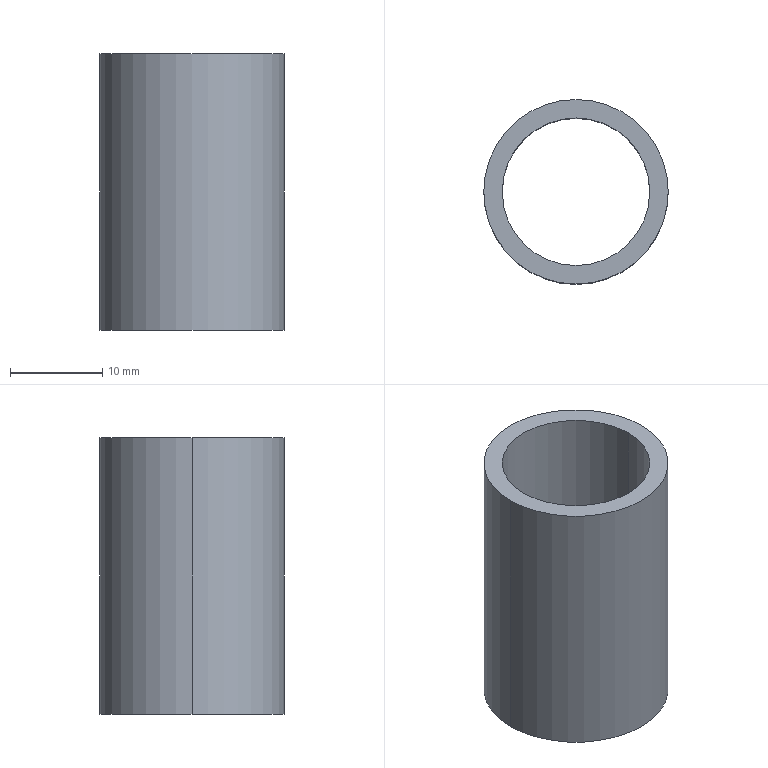Part | SolidWorks | features ExtruThin 1 | 1 solid | 6 faces | box 20 x 20 x 30 mm | volume 3393 mm3 | cylinder 4 | plane 2 | commonest cylinder face diameters 16 x2 20 x2
STEP:
#1=CARTESIAN_POINT('',(-8.,0.,30.));
#2=VERTEX_POINT('',#1);
#3=CARTESIAN_POINT('',(8.,0.,30.));
#4=VERTEX_POINT('',#3);
#5=CARTESIAN_POINT('',(0.,0.,30.));
#6=DIRECTION('',(0.,0.,1.));
#7=DIRECTION('',(1.,0.,0.));
#8=AXIS2_PLACEMENT_3D('',#5,#6,#7);
#9=CIRCLE('',#8,8.);
#10=EDGE_CURVE('',#2,#4,#9,.T.);
#11=ORIENTED_EDGE('',*,*,#10,.T.);
#12=CARTESIAN_POINT('',(8.,0.,0.));
#13=VERTEX_POINT('',#12);
#14=CARTESIAN_POINT('',(8.,0.,30.));
#15=DIRECTION('',(0.,0.,-1.));
#16=VECTOR('',#15,1000.);
#17=LINE('',#14,#16);
#18=EDGE_CURVE('',#4,#13,#17,.T.);
#19=ORIENTED_EDGE('',*,*,#18,.T.);
#20=CARTESIAN_POINT('',(-8.,0.,0.));
#21=VERTEX_POINT('',#20);
#22=CARTESIAN_POINT('',(0.,0.,0.));
#23=DIRECTION('',(0.,0.,1.));
#24=DIRECTION('',(1.,0.,0.));
#25=AXIS2_PLACEMENT_3D('',#22,#23,#24);
#26=CIRCLE('',#25,8.);
#27=EDGE_CURVE('',#21,#13,#26,.T.);
#28=ORIENTED_EDGE('',*,*,#27,.F.);
#29=CARTESIAN_POINT('',(-8.,0.,30.));
#30=DIRECTION('',(0.,0.,-1.));
#31=VECTOR('',#30,1000.);
#32=LINE('',#29,#31);
#33=EDGE_CURVE('',#2,#21,#32,.T.);
#34=ORIENTED_EDGE('',*,*,#33,.F.);
#35=EDGE_LOOP('',(#11,#19,#28,#34));
#36=FACE_OUTER_BOUND('',#35,.T.);
#37=CARTESIAN_POINT('',(0.,0.,30.));
#38=DIRECTION('',(0.,0.,-1.));
#39=DIRECTION('',(-1.,0.,0.));
#40=AXIS2_PLACEMENT_3D('',#37,#38,#39);
#41=CYLINDRICAL_SURFACE('',#40,8.);
#42=ADVANCED_FACE('',(#36),#41,.F.);
#43=CARTESIAN_POINT('',(10.,0.,30.));
#44=VERTEX_POINT('',#43);
#45=CARTESIAN_POINT('',(-10.,0.,30.));
#46=VERTEX_POINT('',#45);
#47=CARTESIAN_POINT('',(0.,0.,30.));
#48=DIRECTION('',(0.,0.,1.));
#49=DIRECTION('',(1.,0.,0.));
#50=AXIS2_PLACEMENT_3D('',#47,#48,#49);
#51=CIRCLE('',#50,10.);
#52=EDGE_CURVE('',#44,#46,#51,.T.);
#53=ORIENTED_EDGE('',*,*,#52,.F.);
#54=CARTESIAN_POINT('',(10.,0.,0.));
#55=VERTEX_POINT('',#54);
#56=CARTESIAN_POINT('',(10.,0.,30.));
#57=DIRECTION('',(0.,0.,-1.));
#58=VECTOR('',#57,1000.);
#59=LINE('',#56,#58);
#60=EDGE_CURVE('',#44,#55,#59,.T.);
#61=ORIENTED_EDGE('',*,*,#60,.T.);
#62=CARTESIAN_POINT('',(-10.,0.,0.));
#63=VERTEX_POINT('',#62);
#64=CARTESIAN_POINT('',(0.,0.,0.));
#65=DIRECTION('',(0.,0.,1.));
#66=DIRECTION('',(1.,0.,0.));
#67=AXIS2_PLACEMENT_3D('',#64,#65,#66);
#68=CIRCLE('',#67,10.);
#69=EDGE_CURVE('',#55,#63,#68,.T.);
#70=ORIENTED_EDGE('',*,*,#69,.T.);
#71=CARTESIAN_POINT('',(-10.,0.,30.));
#72=DIRECTION('',(0.,0.,-1.));
#73=VECTOR('',#72,1000.);
#74=LINE('',#71,#73);
#75=EDGE_CURVE('',#46,#63,#74,.T.);
#76=ORIENTED_EDGE('',*,*,#75,.F.);
#77=EDGE_LOOP('',(#53,#61,#70,#76));
#78=FACE_OUTER_BOUND('',#77,.T.);
#79=CARTESIAN_POINT('',(0.,0.,30.));
#80=DIRECTION('',(0.,0.,-1.));
#81=DIRECTION('',(-1.,0.,0.));
#82=AXIS2_PLACEMENT_3D('',#79,#80,#81);
#83=CYLINDRICAL_SURFACE('',#82,10.);
#84=ADVANCED_FACE('',(#78),#83,.T.);
#85=CARTESIAN_POINT('',(0.,0.,30.));
#86=DIRECTION('',(0.,0.,1.));
#87=DIRECTION('',(1.,0.,0.));
#88=AXIS2_PLACEMENT_3D('',#85,#86,#87);
#89=CIRCLE('',#88,10.);
#90=EDGE_CURVE('',#46,#44,#89,.T.);
#91=ORIENTED_EDGE('',*,*,#90,.T.);
#92=ORIENTED_EDGE('',*,*,#52,.T.);
#93=EDGE_LOOP('',(#91,#92));
#94=FACE_OUTER_BOUND('',#93,.T.);
#95=ORIENTED_EDGE('',*,*,#10,.F.);
#96=CARTESIAN_POINT('',(0.,0.,30.));
#97=DIRECTION('',(0.,0.,1.));
#98=DIRECTION('',(1.,0.,0.));
#99=AXIS2_PLACEMENT_3D('',#96,#97,#98);
#100=CIRCLE('',#99,8.);
#101=EDGE_CURVE('',#4,#2,#100,.T.);
#102=ORIENTED_EDGE('',*,*,#101,.F.);
#103=EDGE_LOOP('',(#95,#102));
#104=FACE_BOUND('',#103,.T.);
#105=CARTESIAN_POINT('',(0.,0.,30.));
#106=DIRECTION('',(0.,0.,1.));
#107=DIRECTION('',(1.,0.,0.));
#108=AXIS2_PLACEMENT_3D('',#105,#106,#107);
#109=PLANE('',#108);
#110=ADVANCED_FACE('',(#94,#104),#109,.T.);
#111=CARTESIAN_POINT('',(0.,0.,0.));
#112=DIRECTION('',(0.,0.,1.));
#113=DIRECTION('',(1.,0.,0.));
#114=AXIS2_PLACEMENT_3D('',#111,#112,#113);
#115=CIRCLE('',#114,10.);
#116=EDGE_CURVE('',#63,#55,#115,.T.);
#117=ORIENTED_EDGE('',*,*,#116,.F.);
#118=ORIENTED_EDGE('',*,*,#69,.F.);
#119=EDGE_LOOP('',(#117,#118));
#120=FACE_OUTER_BOUND('',#119,.T.);
#121=ORIENTED_EDGE('',*,*,#27,.T.);
#122=CARTESIAN_POINT('',(0.,0.,0.));
#123=DIRECTION('',(0.,0.,1.));
#124=DIRECTION('',(1.,0.,0.));
#125=AXIS2_PLACEMENT_3D('',#122,#123,#124);
#126=CIRCLE('',#125,8.);
#127=EDGE_CURVE('',#13,#21,#126,.T.);
#128=ORIENTED_EDGE('',*,*,#127,.T.);
#129=EDGE_LOOP('',(#121,#128));
#130=FACE_BOUND('',#129,.T.);
#131=CARTESIAN_POINT('',(0.,0.,0.));
#132=DIRECTION('',(0.,0.,1.));
#133=DIRECTION('',(1.,0.,0.));
#134=AXIS2_PLACEMENT_3D('',#131,#132,#133);
#135=PLANE('',#134);
#136=ADVANCED_FACE('',(#120,#130),#135,.F.);
#137=ORIENTED_EDGE('',*,*,#60,.F.);
#138=ORIENTED_EDGE('',*,*,#90,.F.);
#139=ORIENTED_EDGE('',*,*,#75,.T.);
#140=ORIENTED_EDGE('',*,*,#116,.T.);
#141=EDGE_LOOP('',(#137,#138,#139,#140));
#142=FACE_OUTER_BOUND('',#141,.T.);
#143=CARTESIAN_POINT('',(0.,0.,30.));
#144=DIRECTION('',(0.,0.,-1.));
#145=DIRECTION('',(-1.,0.,0.));
#146=AXIS2_PLACEMENT_3D('',#143,#144,#145);
#147=CYLINDRICAL_SURFACE('',#146,10.);
#148=ADVANCED_FACE('',(#142),#147,.T.);
#149=ORIENTED_EDGE('',*,*,#18,.F.);
#150=ORIENTED_EDGE('',*,*,#101,.T.);
#151=ORIENTED_EDGE('',*,*,#33,.T.);
#152=ORIENTED_EDGE('',*,*,#127,.F.);
#153=EDGE_LOOP('',(#149,#150,#151,#152));
#154=FACE_OUTER_BOUND('',#153,.T.);
#155=CARTESIAN_POINT('',(0.,0.,30.));
#156=DIRECTION('',(0.,0.,-1.));
#157=DIRECTION('',(-1.,0.,0.));
#158=AXIS2_PLACEMENT_3D('',#155,#156,#157);
#159=CYLINDRICAL_SURFACE('',#158,8.);
#160=ADVANCED_FACE('',(#154),#159,.F.);
#161=CLOSED_SHELL('',(#42,#84,#110,#136,#148,#160));
#162=MANIFOLD_SOLID_BREP('',#161);
#163=CARTESIAN_POINT('',(0.,0.,0.));
#164=DIRECTION('',(0.,0.,1.));
#165=DIRECTION('',(1.,0.,0.));
#166=AXIS2_PLACEMENT_3D('',#163,#164,#165);
#167=(LENGTH_UNIT()NAMED_UNIT(*)SI_UNIT(.MILLI.,.METRE.));
#168=UNCERTAINTY_MEASURE_WITH_UNIT(LENGTH_MEASURE(0.00001),#167,'','');
#169=(NAMED_UNIT(*)PLANE_ANGLE_UNIT()SI_UNIT($,.RADIAN.));
#170=(NAMED_UNIT(*)SI_UNIT($,.STERADIAN.)SOLID_ANGLE_UNIT());
#171=(GEOMETRIC_REPRESENTATION_CONTEXT(3)GLOBAL_UNCERTAINTY_ASSIGNED_CONTEXT((#168))GLOBAL_UNIT_ASSIGNED_CONTEXT((#167,#169,#170))REPRESENTATION_CONTEXT('',''));
#172=ADVANCED_BREP_SHAPE_REPRESENTATION('',(#162,#166),#171);